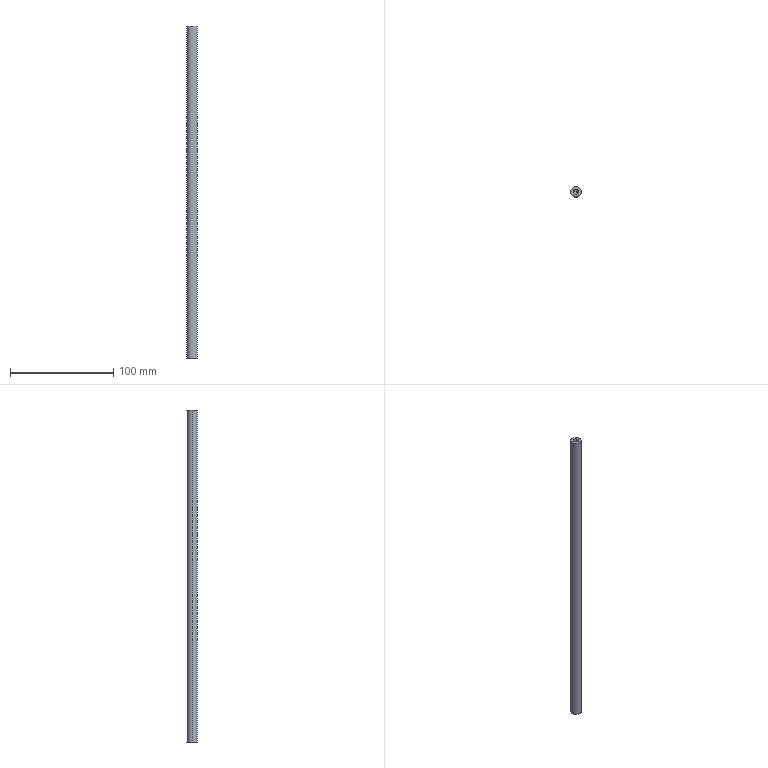Part | SolidWorks | features HoleWzd 2, Extrusion 1 | 1 solid | 12 faces | box 10 x 10 x 321 mm | volume 24603 mm3 | cylinder 6 | cone 4 | plane 2 | commonest cylinder face diameters 5 x4 10 x2
STEP:
#1=CARTESIAN_POINT('',(2.5,0.,15.));
#2=VERTEX_POINT('',#1);
#3=CARTESIAN_POINT('',(-2.5,0.,15.));
#4=VERTEX_POINT('',#3);
#5=CARTESIAN_POINT('',(0.,0.,15.));
#6=DIRECTION('',(0.,0.,-1.));
#7=DIRECTION('',(-1.,0.,0.));
#8=AXIS2_PLACEMENT_3D('',#5,#6,#7);
#9=CIRCLE('',#8,2.5);
#10=EDGE_CURVE('',#2,#4,#9,.T.);
#11=ORIENTED_EDGE('',*,*,#10,.F.);
#12=CARTESIAN_POINT('',(2.5,0.,0.));
#13=VERTEX_POINT('',#12);
#14=CARTESIAN_POINT('',(2.5,0.,0.));
#15=DIRECTION('',(0.,0.,-1.));
#16=VECTOR('',#15,1000.);
#17=LINE('',#14,#16);
#18=EDGE_CURVE('',#2,#13,#17,.T.);
#19=ORIENTED_EDGE('',*,*,#18,.T.);
#20=CARTESIAN_POINT('',(-2.5,0.,0.));
#21=VERTEX_POINT('',#20);
#22=CARTESIAN_POINT('',(0.,0.,0.));
#23=DIRECTION('',(0.,0.,-1.));
#24=DIRECTION('',(-1.,0.,0.));
#25=AXIS2_PLACEMENT_3D('',#22,#23,#24);
#26=CIRCLE('',#25,2.5);
#27=EDGE_CURVE('',#13,#21,#26,.T.);
#28=ORIENTED_EDGE('',*,*,#27,.T.);
#29=CARTESIAN_POINT('',(-2.5,0.,0.));
#30=DIRECTION('',(0.,0.,-1.));
#31=VECTOR('',#30,1000.);
#32=LINE('',#29,#31);
#33=EDGE_CURVE('',#4,#21,#32,.T.);
#34=ORIENTED_EDGE('',*,*,#33,.F.);
#35=EDGE_LOOP('',(#11,#19,#28,#34));
#36=FACE_OUTER_BOUND('',#35,.T.);
#37=CARTESIAN_POINT('',(0.,0.,0.));
#38=DIRECTION('',(0.,0.,-1.));
#39=DIRECTION('',(-1.,0.,0.));
#40=AXIS2_PLACEMENT_3D('',#37,#38,#39);
#41=CYLINDRICAL_SURFACE('',#40,2.5);
#42=ADVANCED_FACE('',(#36),#41,.F.);
#43=CARTESIAN_POINT('',(0.,0.,16.502));
#44=VERTEX_POINT('',#43);
#45=CARTESIAN_POINT('',(-2.5,0.,15.));
#46=DIRECTION('',(-0.8572,0.,-0.515));
#47=VECTOR('',#46,1000.);
#48=LINE('',#45,#47);
#49=EDGE_CURVE('',#44,#4,#48,.T.);
#50=ORIENTED_EDGE('',*,*,#49,.F.);
#51=CARTESIAN_POINT('',(2.5,0.,15.));
#52=DIRECTION('',(0.8572,0.,-0.515));
#53=VECTOR('',#52,1000.);
#54=LINE('',#51,#53);
#55=EDGE_CURVE('',#44,#2,#54,.T.);
#56=ORIENTED_EDGE('',*,*,#55,.T.);
#57=ORIENTED_EDGE('',*,*,#10,.T.);
#58=EDGE_LOOP('',(#50,#56,#57));
#59=FACE_OUTER_BOUND('',#58,.T.);
#60=CARTESIAN_POINT('',(0.,0.,15.));
#61=DIRECTION('',(0.,0.,-1.));
#62=DIRECTION('',(-1.,0.,0.));
#63=AXIS2_PLACEMENT_3D('',#60,#61,#62);
#64=CONICAL_SURFACE('',#63,2.5,1.03);
#65=ADVANCED_FACE('',(#59),#64,.F.);
#66=CARTESIAN_POINT('',(-2.5,0.,306.));
#67=VERTEX_POINT('',#66);
#68=CARTESIAN_POINT('',(2.5,0.,306.));
#69=VERTEX_POINT('',#68);
#70=CARTESIAN_POINT('',(0.,0.,306.));
#71=DIRECTION('',(0.,0.,1.));
#72=DIRECTION('',(1.,0.,0.));
#73=AXIS2_PLACEMENT_3D('',#70,#71,#72);
#74=CIRCLE('',#73,2.5);
#75=EDGE_CURVE('',#67,#69,#74,.T.);
#76=ORIENTED_EDGE('',*,*,#75,.F.);
#77=CARTESIAN_POINT('',(-2.5,0.,321.));
#78=VERTEX_POINT('',#77);
#79=CARTESIAN_POINT('',(-2.5,0.,321.));
#80=DIRECTION('',(0.,0.,1.));
#81=VECTOR('',#80,1000.);
#82=LINE('',#79,#81);
#83=EDGE_CURVE('',#67,#78,#82,.T.);
#84=ORIENTED_EDGE('',*,*,#83,.T.);
#85=CARTESIAN_POINT('',(2.5,0.,321.));
#86=VERTEX_POINT('',#85);
#87=CARTESIAN_POINT('',(0.,0.,321.));
#88=DIRECTION('',(0.,0.,1.));
#89=DIRECTION('',(1.,0.,0.));
#90=AXIS2_PLACEMENT_3D('',#87,#88,#89);
#91=CIRCLE('',#90,2.5);
#92=EDGE_CURVE('',#78,#86,#91,.T.);
#93=ORIENTED_EDGE('',*,*,#92,.T.);
#94=CARTESIAN_POINT('',(2.5,0.,321.));
#95=DIRECTION('',(0.,0.,1.));
#96=VECTOR('',#95,1000.);
#97=LINE('',#94,#96);
#98=EDGE_CURVE('',#69,#86,#97,.T.);
#99=ORIENTED_EDGE('',*,*,#98,.F.);
#100=EDGE_LOOP('',(#76,#84,#93,#99));
#101=FACE_OUTER_BOUND('',#100,.T.);
#102=CARTESIAN_POINT('',(0.,0.,321.));
#103=DIRECTION('',(0.,0.,1.));
#104=DIRECTION('',(1.,0.,0.));
#105=AXIS2_PLACEMENT_3D('',#102,#103,#104);
#106=CYLINDRICAL_SURFACE('',#105,2.5);
#107=ADVANCED_FACE('',(#101),#106,.F.);
#108=CARTESIAN_POINT('',(0.,0.,304.498));
#109=VERTEX_POINT('',#108);
#110=CARTESIAN_POINT('',(2.5,0.,306.));
#111=DIRECTION('',(0.8572,0.,0.515));
#112=VECTOR('',#111,1000.);
#113=LINE('',#110,#112);
#114=EDGE_CURVE('',#109,#69,#113,.T.);
#115=ORIENTED_EDGE('',*,*,#114,.F.);
#116=CARTESIAN_POINT('',(-2.5,0.,306.));
#117=DIRECTION('',(-0.8572,0.,0.515));
#118=VECTOR('',#117,1000.);
#119=LINE('',#116,#118);
#120=EDGE_CURVE('',#109,#67,#119,.T.);
#121=ORIENTED_EDGE('',*,*,#120,.T.);
#122=ORIENTED_EDGE('',*,*,#75,.T.);
#123=EDGE_LOOP('',(#115,#121,#122));
#124=FACE_OUTER_BOUND('',#123,.T.);
#125=CARTESIAN_POINT('',(0.,0.,306.));
#126=DIRECTION('',(0.,0.,1.));
#127=DIRECTION('',(1.,0.,0.));
#128=AXIS2_PLACEMENT_3D('',#125,#126,#127);
#129=CONICAL_SURFACE('',#128,2.5,1.03);
#130=ADVANCED_FACE('',(#124),#129,.F.);
#131=CARTESIAN_POINT('',(5.,0.,321.));
#132=VERTEX_POINT('',#131);
#133=CARTESIAN_POINT('',(-5.,0.,321.));
#134=VERTEX_POINT('',#133);
#135=CARTESIAN_POINT('',(0.,0.,321.));
#136=DIRECTION('',(0.,0.,1.));
#137=DIRECTION('',(1.,0.,0.));
#138=AXIS2_PLACEMENT_3D('',#135,#136,#137);
#139=CIRCLE('',#138,5.);
#140=EDGE_CURVE('',#132,#134,#139,.T.);
#141=ORIENTED_EDGE('',*,*,#140,.F.);
#142=CARTESIAN_POINT('',(5.,0.,0.));
#143=VERTEX_POINT('',#142);
#144=CARTESIAN_POINT('',(5.,0.,321.));
#145=DIRECTION('',(0.,0.,-1.));
#146=VECTOR('',#145,1000.);
#147=LINE('',#144,#146);
#148=EDGE_CURVE('',#132,#143,#147,.T.);
#149=ORIENTED_EDGE('',*,*,#148,.T.);
#150=CARTESIAN_POINT('',(-5.,0.,0.));
#151=VERTEX_POINT('',#150);
#152=CARTESIAN_POINT('',(0.,0.,0.));
#153=DIRECTION('',(0.,0.,1.));
#154=DIRECTION('',(1.,0.,0.));
#155=AXIS2_PLACEMENT_3D('',#152,#153,#154);
#156=CIRCLE('',#155,5.);
#157=EDGE_CURVE('',#143,#151,#156,.T.);
#158=ORIENTED_EDGE('',*,*,#157,.T.);
#159=CARTESIAN_POINT('',(-5.,0.,321.));
#160=DIRECTION('',(0.,0.,-1.));
#161=VECTOR('',#160,1000.);
#162=LINE('',#159,#161);
#163=EDGE_CURVE('',#134,#151,#162,.T.);
#164=ORIENTED_EDGE('',*,*,#163,.F.);
#165=EDGE_LOOP('',(#141,#149,#158,#164));
#166=FACE_OUTER_BOUND('',#165,.T.);
#167=CARTESIAN_POINT('',(0.,0.,321.));
#168=DIRECTION('',(0.,0.,-1.));
#169=DIRECTION('',(-1.,0.,0.));
#170=AXIS2_PLACEMENT_3D('',#167,#168,#169);
#171=CYLINDRICAL_SURFACE('',#170,5.);
#172=ADVANCED_FACE('',(#166),#171,.T.);
#173=ORIENTED_EDGE('',*,*,#148,.F.);
#174=CARTESIAN_POINT('',(0.,0.,321.));
#175=DIRECTION('',(0.,0.,1.));
#176=DIRECTION('',(1.,0.,0.));
#177=AXIS2_PLACEMENT_3D('',#174,#175,#176);
#178=CIRCLE('',#177,5.);
#179=EDGE_CURVE('',#134,#132,#178,.T.);
#180=ORIENTED_EDGE('',*,*,#179,.F.);
#181=ORIENTED_EDGE('',*,*,#163,.T.);
#182=CARTESIAN_POINT('',(0.,0.,0.));
#183=DIRECTION('',(0.,0.,1.));
#184=DIRECTION('',(1.,0.,0.));
#185=AXIS2_PLACEMENT_3D('',#182,#183,#184);
#186=CIRCLE('',#185,5.);
#187=EDGE_CURVE('',#151,#143,#186,.T.);
#188=ORIENTED_EDGE('',*,*,#187,.T.);
#189=EDGE_LOOP('',(#173,#180,#181,#188));
#190=FACE_OUTER_BOUND('',#189,.T.);
#191=CARTESIAN_POINT('',(0.,0.,321.));
#192=DIRECTION('',(0.,0.,-1.));
#193=DIRECTION('',(-1.,0.,0.));
#194=AXIS2_PLACEMENT_3D('',#191,#192,#193);
#195=CYLINDRICAL_SURFACE('',#194,5.);
#196=ADVANCED_FACE('',(#190),#195,.T.);
#197=CARTESIAN_POINT('',(0.,0.,321.));
#198=DIRECTION('',(0.,0.,1.));
#199=DIRECTION('',(1.,0.,0.));
#200=AXIS2_PLACEMENT_3D('',#197,#198,#199);
#201=CIRCLE('',#200,2.5);
#202=EDGE_CURVE('',#86,#78,#201,.T.);
#203=ORIENTED_EDGE('',*,*,#202,.F.);
#204=ORIENTED_EDGE('',*,*,#92,.F.);
#205=EDGE_LOOP('',(#203,#204));
#206=FACE_BOUND('',#205,.T.);
#207=ORIENTED_EDGE('',*,*,#179,.T.);
#208=ORIENTED_EDGE('',*,*,#140,.T.);
#209=EDGE_LOOP('',(#207,#208));
#210=FACE_OUTER_BOUND('',#209,.T.);
#211=CARTESIAN_POINT('',(0.,0.,321.));
#212=DIRECTION('',(0.,0.,1.));
#213=DIRECTION('',(1.,0.,0.));
#214=AXIS2_PLACEMENT_3D('',#211,#212,#213);
#215=PLANE('',#214);
#216=ADVANCED_FACE('',(#206,#210),#215,.T.);
#217=CARTESIAN_POINT('',(0.,0.,0.));
#218=DIRECTION('',(0.,0.,-1.));
#219=DIRECTION('',(-1.,0.,0.));
#220=AXIS2_PLACEMENT_3D('',#217,#218,#219);
#221=CIRCLE('',#220,2.5);
#222=EDGE_CURVE('',#21,#13,#221,.T.);
#223=ORIENTED_EDGE('',*,*,#222,.F.);
#224=ORIENTED_EDGE('',*,*,#27,.F.);
#225=EDGE_LOOP('',(#223,#224));
#226=FACE_BOUND('',#225,.T.);
#227=ORIENTED_EDGE('',*,*,#187,.F.);
#228=ORIENTED_EDGE('',*,*,#157,.F.);
#229=EDGE_LOOP('',(#227,#228));
#230=FACE_OUTER_BOUND('',#229,.T.);
#231=CARTESIAN_POINT('',(0.,0.,0.));
#232=DIRECTION('',(0.,0.,1.));
#233=DIRECTION('',(1.,0.,0.));
#234=AXIS2_PLACEMENT_3D('',#231,#232,#233);
#235=PLANE('',#234);
#236=ADVANCED_FACE('',(#226,#230),#235,.F.);
#237=ORIENTED_EDGE('',*,*,#120,.F.);
#238=ORIENTED_EDGE('',*,*,#114,.T.);
#239=CARTESIAN_POINT('',(0.,0.,306.));
#240=DIRECTION('',(0.,0.,1.));
#241=DIRECTION('',(1.,0.,0.));
#242=AXIS2_PLACEMENT_3D('',#239,#240,#241);
#243=CIRCLE('',#242,2.5);
#244=EDGE_CURVE('',#69,#67,#243,.T.);
#245=ORIENTED_EDGE('',*,*,#244,.T.);
#246=EDGE_LOOP('',(#237,#238,#245));
#247=FACE_OUTER_BOUND('',#246,.T.);
#248=CARTESIAN_POINT('',(0.,0.,306.));
#249=DIRECTION('',(0.,0.,1.));
#250=DIRECTION('',(1.,0.,0.));
#251=AXIS2_PLACEMENT_3D('',#248,#249,#250);
#252=CONICAL_SURFACE('',#251,2.5,1.03);
#253=ADVANCED_FACE('',(#247),#252,.F.);
#254=ORIENTED_EDGE('',*,*,#83,.F.);
#255=ORIENTED_EDGE('',*,*,#244,.F.);
#256=ORIENTED_EDGE('',*,*,#98,.T.);
#257=ORIENTED_EDGE('',*,*,#202,.T.);
#258=EDGE_LOOP('',(#254,#255,#256,#257));
#259=FACE_OUTER_BOUND('',#258,.T.);
#260=CARTESIAN_POINT('',(0.,0.,321.));
#261=DIRECTION('',(0.,0.,1.));
#262=DIRECTION('',(1.,0.,0.));
#263=AXIS2_PLACEMENT_3D('',#260,#261,#262);
#264=CYLINDRICAL_SURFACE('',#263,2.5);
#265=ADVANCED_FACE('',(#259),#264,.F.);
#266=ORIENTED_EDGE('',*,*,#55,.F.);
#267=ORIENTED_EDGE('',*,*,#49,.T.);
#268=CARTESIAN_POINT('',(0.,0.,15.));
#269=DIRECTION('',(0.,0.,-1.));
#270=DIRECTION('',(-1.,0.,0.));
#271=AXIS2_PLACEMENT_3D('',#268,#269,#270);
#272=CIRCLE('',#271,2.5);
#273=EDGE_CURVE('',#4,#2,#272,.T.);
#274=ORIENTED_EDGE('',*,*,#273,.T.);
#275=EDGE_LOOP('',(#266,#267,#274));
#276=FACE_OUTER_BOUND('',#275,.T.);
#277=CARTESIAN_POINT('',(0.,0.,15.));
#278=DIRECTION('',(0.,0.,-1.));
#279=DIRECTION('',(-1.,0.,0.));
#280=AXIS2_PLACEMENT_3D('',#277,#278,#279);
#281=CONICAL_SURFACE('',#280,2.5,1.03);
#282=ADVANCED_FACE('',(#276),#281,.F.);
#283=ORIENTED_EDGE('',*,*,#18,.F.);
#284=ORIENTED_EDGE('',*,*,#273,.F.);
#285=ORIENTED_EDGE('',*,*,#33,.T.);
#286=ORIENTED_EDGE('',*,*,#222,.T.);
#287=EDGE_LOOP('',(#283,#284,#285,#286));
#288=FACE_OUTER_BOUND('',#287,.T.);
#289=CARTESIAN_POINT('',(0.,0.,0.));
#290=DIRECTION('',(0.,0.,-1.));
#291=DIRECTION('',(-1.,0.,0.));
#292=AXIS2_PLACEMENT_3D('',#289,#290,#291);
#293=CYLINDRICAL_SURFACE('',#292,2.5);
#294=ADVANCED_FACE('',(#288),#293,.F.);
#295=CLOSED_SHELL('',(#42,#65,#107,#130,#172,#196,#216,#236,#253,#265,#282,#294));
#296=MANIFOLD_SOLID_BREP('',#295);
#297=CARTESIAN_POINT('',(0.,0.,0.));
#298=DIRECTION('',(0.,0.,1.));
#299=DIRECTION('',(1.,0.,0.));
#300=AXIS2_PLACEMENT_3D('',#297,#298,#299);
#301=(LENGTH_UNIT()NAMED_UNIT(*)SI_UNIT(.MILLI.,.METRE.));
#302=UNCERTAINTY_MEASURE_WITH_UNIT(LENGTH_MEASURE(0.00001),#301,'','');
#303=(NAMED_UNIT(*)PLANE_ANGLE_UNIT()SI_UNIT($,.RADIAN.));
#304=(NAMED_UNIT(*)SI_UNIT($,.STERADIAN.)SOLID_ANGLE_UNIT());
#305=(GEOMETRIC_REPRESENTATION_CONTEXT(3)GLOBAL_UNCERTAINTY_ASSIGNED_CONTEXT((#302))GLOBAL_UNIT_ASSIGNED_CONTEXT((#301,#303,#304))REPRESENTATION_CONTEXT('',''));
#306=ADVANCED_BREP_SHAPE_REPRESENTATION('',(#296,#300),#305);